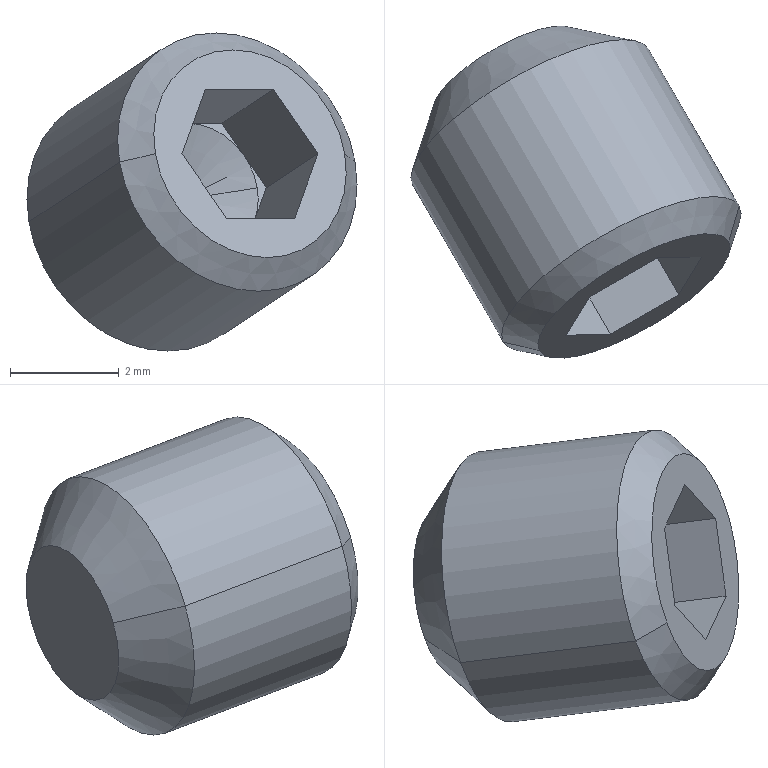Part | SolidWorks | features BaseBody 1 | 1 solid | 22 faces | box 6.067 x 6.109 x 5.848 mm | volume 77.596 mm3 | plane 14 | cone 6 | cylinder 2 | commonest cylinder face diameters 5 x2
STEP:
#1=CARTESIAN_POINT('',(451.556,1814.827,-1176.378));
#2=VERTEX_POINT('',#1);
#3=CARTESIAN_POINT('',(447.226,1812.327,-1176.378));
#4=VERTEX_POINT('',#3);
#5=CARTESIAN_POINT('',(449.391,1813.577,-1176.378));
#6=DIRECTION('',(0.4749,-0.8225,0.3132));
#7=DIRECTION('',(0.866,0.5,0.));
#8=AXIS2_PLACEMENT_3D('',#5,#6,#7);
#9=CIRCLE('',#8,2.5);
#10=EDGE_CURVE('',#2,#4,#9,.T.);
#11=ORIENTED_EDGE('',*,*,#10,.T.);
#12=CARTESIAN_POINT('',(448.893,1809.44,-1175.279));
#13=VERTEX_POINT('',#12);
#14=CARTESIAN_POINT('',(449.126,1809.037,-1175.125));
#15=DIRECTION('',(0.4749,-0.8225,0.3132));
#16=VECTOR('',#15,1000.);
#17=LINE('',#14,#16);
#18=EDGE_CURVE('',#4,#13,#17,.T.);
#19=ORIENTED_EDGE('',*,*,#18,.T.);
#20=CARTESIAN_POINT('',(453.223,1811.94,-1175.279));
#21=VERTEX_POINT('',#20);
#22=CARTESIAN_POINT('',(451.058,1810.69,-1175.279));
#23=DIRECTION('',(-0.4749,0.8225,-0.3132));
#24=DIRECTION('',(0.866,0.5,0.));
#25=AXIS2_PLACEMENT_3D('',#22,#23,#24);
#26=CIRCLE('',#25,2.5);
#27=EDGE_CURVE('',#13,#21,#26,.T.);
#28=ORIENTED_EDGE('',*,*,#27,.T.);
#29=CARTESIAN_POINT('',(453.456,1811.537,-1175.125));
#30=DIRECTION('',(0.4749,-0.8225,0.3132));
#31=VECTOR('',#30,1000.);
#32=LINE('',#29,#31);
#33=EDGE_CURVE('',#2,#21,#32,.T.);
#34=ORIENTED_EDGE('',*,*,#33,.F.);
#35=EDGE_LOOP('',(#11,#19,#28,#34));
#36=FACE_OUTER_BOUND('',#35,.T.);
#37=CARTESIAN_POINT('',(451.291,1810.287,-1175.125));
#38=DIRECTION('',(0.4749,-0.8225,0.3132));
#39=DIRECTION('',(0.866,0.5,0.));
#40=AXIS2_PLACEMENT_3D('',#37,#38,#39);
#41=CYLINDRICAL_SURFACE('',#40,2.5);
#42=ADVANCED_FACE('',(#36),#41,.T.);
#43=CARTESIAN_POINT('',(449.55,1809.282,-1175.125));
#44=VERTEX_POINT('',#43);
#45=CARTESIAN_POINT('',(453.031,1811.292,-1175.125));
#46=VERTEX_POINT('',#45);
#47=CARTESIAN_POINT('',(451.291,1810.287,-1175.125));
#48=DIRECTION('',(-0.4749,0.8225,-0.3132));
#49=DIRECTION('',(-0.866,-0.5,0.));
#50=AXIS2_PLACEMENT_3D('',#47,#48,#49);
#51=CIRCLE('',#50,2.009);
#52=EDGE_CURVE('',#44,#46,#51,.T.);
#53=ORIENTED_EDGE('',*,*,#52,.T.);
#54=CARTESIAN_POINT('',(453.223,1811.94,-1175.279));
#55=DIRECTION('',(0.2766,0.9351,-0.2214));
#56=VECTOR('',#55,1000.);
#57=LINE('',#54,#56);
#58=EDGE_CURVE('',#46,#21,#57,.T.);
#59=ORIENTED_EDGE('',*,*,#58,.T.);
#60=ORIENTED_EDGE('',*,*,#27,.F.);
#61=CARTESIAN_POINT('',(448.893,1809.44,-1175.279));
#62=DIRECTION('',(-0.9481,0.228,-0.2214));
#63=VECTOR('',#62,1000.);
#64=LINE('',#61,#63);
#65=EDGE_CURVE('',#44,#13,#64,.T.);
#66=ORIENTED_EDGE('',*,*,#65,.F.);
#67=EDGE_LOOP('',(#53,#59,#60,#66));
#68=FACE_OUTER_BOUND('',#67,.T.);
#69=CARTESIAN_POINT('',(451.058,1810.69,-1175.279));
#70=DIRECTION('',(-0.4749,0.8225,-0.3132));
#71=DIRECTION('',(-0.866,-0.5,0.));
#72=AXIS2_PLACEMENT_3D('',#69,#70,#71);
#73=CONICAL_SURFACE('',#72,2.5,0.7854);
#74=ADVANCED_FACE('',(#68),#73,.T.);
#75=CARTESIAN_POINT('',(450.216,1815.149,-1176.691));
#76=VERTEX_POINT('',#75);
#77=CARTESIAN_POINT('',(447.617,1813.649,-1176.691));
#78=VERTEX_POINT('',#77);
#79=CARTESIAN_POINT('',(448.916,1814.399,-1176.691));
#80=DIRECTION('',(0.4749,-0.8225,0.3132));
#81=DIRECTION('',(0.866,0.5,0.));
#82=AXIS2_PLACEMENT_3D('',#79,#80,#81);
#83=CIRCLE('',#82,1.5);
#84=EDGE_CURVE('',#76,#78,#83,.T.);
#85=ORIENTED_EDGE('',*,*,#84,.T.);
#86=CARTESIAN_POINT('',(447.226,1812.327,-1176.378));
#87=DIRECTION('',(-0.2766,-0.9351,0.2214));
#88=VECTOR('',#87,1000.);
#89=LINE('',#86,#88);
#90=EDGE_CURVE('',#78,#4,#89,.T.);
#91=ORIENTED_EDGE('',*,*,#90,.T.);
#92=ORIENTED_EDGE('',*,*,#10,.F.);
#93=CARTESIAN_POINT('',(451.556,1814.827,-1176.378));
#94=DIRECTION('',(0.9481,-0.228,0.2214));
#95=VECTOR('',#94,1000.);
#96=LINE('',#93,#95);
#97=EDGE_CURVE('',#76,#2,#96,.T.);
#98=ORIENTED_EDGE('',*,*,#97,.F.);
#99=EDGE_LOOP('',(#85,#91,#92,#98));
#100=FACE_OUTER_BOUND('',#99,.T.);
#101=CARTESIAN_POINT('',(449.391,1813.577,-1176.378));
#102=DIRECTION('',(0.4749,-0.8225,0.3132));
#103=DIRECTION('',(0.866,0.5,0.));
#104=AXIS2_PLACEMENT_3D('',#101,#102,#103);
#105=CONICAL_SURFACE('',#104,2.5,0.7854);
#106=ADVANCED_FACE('',(#100),#105,.T.);
#107=CARTESIAN_POINT('',(449.998,1812.525,-1175.978));
#108=VERTEX_POINT('',#107);
#109=CARTESIAN_POINT('',(451.424,1812.557,-1175.752));
#110=VERTEX_POINT('',#109);
#111=CARTESIAN_POINT('',(451.424,1812.557,-1175.752));
#112=DIRECTION('',(0.9874,0.02178,0.1566));
#113=VECTOR('',#112,1000.);
#114=LINE('',#111,#113);
#115=EDGE_CURVE('',#108,#110,#114,.T.);
#116=ORIENTED_EDGE('',*,*,#115,.F.);
#117=CARTESIAN_POINT('',(449.258,1811.307,-1175.752));
#118=VERTEX_POINT('',#117);
#119=CARTESIAN_POINT('',(449.258,1811.307,-1175.752));
#120=DIRECTION('',(-0.5126,-0.8442,0.1566));
#121=VECTOR('',#120,1000.);
#122=LINE('',#119,#121);
#123=EDGE_CURVE('',#108,#118,#122,.T.);
#124=ORIENTED_EDGE('',*,*,#123,.T.);
#125=CARTESIAN_POINT('',(449.501,1811.221,-1176.345));
#126=VERTEX_POINT('',#125);
#127=CARTESIAN_POINT('',(450.341,1811.932,-1175.752));
#128=DIRECTION('',(-0.4749,0.8225,-0.3132));
#129=DIRECTION('',(0.866,0.5,0.));
#130=AXIS2_PLACEMENT_3D('',#127,#128,#129);
#131=CIRCLE('',#130,1.25);
#132=EDGE_CURVE('',#126,#118,#131,.T.);
#133=ORIENTED_EDGE('',*,*,#132,.F.);
#134=CARTESIAN_POINT('',(450.537,1811.593,-1176.939));
#135=VERTEX_POINT('',#134);
#136=CARTESIAN_POINT('',(450.341,1811.932,-1175.752));
#137=DIRECTION('',(-0.4749,0.8225,-0.3132));
#138=DIRECTION('',(0.866,0.5,0.));
#139=AXIS2_PLACEMENT_3D('',#136,#137,#138);
#140=CIRCLE('',#139,1.25);
#141=EDGE_CURVE('',#135,#126,#140,.T.);
#142=ORIENTED_EDGE('',*,*,#141,.F.);
#143=CARTESIAN_POINT('',(451.376,1812.304,-1176.345));
#144=VERTEX_POINT('',#143);
#145=CARTESIAN_POINT('',(450.341,1811.932,-1175.752));
#146=DIRECTION('',(-0.4749,0.8225,-0.3132));
#147=DIRECTION('',(0.866,0.5,0.));
#148=AXIS2_PLACEMENT_3D('',#145,#146,#147);
#149=CIRCLE('',#148,1.25);
#150=EDGE_CURVE('',#144,#135,#149,.T.);
#151=ORIENTED_EDGE('',*,*,#150,.F.);
#152=CARTESIAN_POINT('',(450.341,1811.932,-1175.752));
#153=DIRECTION('',(-0.4749,0.8225,-0.3132));
#154=DIRECTION('',(0.866,0.5,0.));
#155=AXIS2_PLACEMENT_3D('',#152,#153,#154);
#156=CIRCLE('',#155,1.25);
#157=EDGE_CURVE('',#110,#144,#156,.T.);
#158=ORIENTED_EDGE('',*,*,#157,.F.);
#159=EDGE_LOOP('',(#116,#124,#133,#142,#151,#158));
#160=FACE_OUTER_BOUND('',#159,.T.);
#161=CARTESIAN_POINT('',(450.341,1811.932,-1175.752));
#162=DIRECTION('',(0.4749,-0.8225,0.3132));
#163=DIRECTION('',(0.866,0.5,0.));
#164=AXIS2_PLACEMENT_3D('',#161,#162,#163);
#165=CONICAL_SURFACE('',#164,1.25,1.047);
#166=ADVANCED_FACE('',(#160),#165,.F.);
#167=ORIENTED_EDGE('',*,*,#18,.F.);
#168=CARTESIAN_POINT('',(449.391,1813.577,-1176.378));
#169=DIRECTION('',(0.4749,-0.8225,0.3132));
#170=DIRECTION('',(0.866,0.5,0.));
#171=AXIS2_PLACEMENT_3D('',#168,#169,#170);
#172=CIRCLE('',#171,2.5);
#173=EDGE_CURVE('',#4,#2,#172,.T.);
#174=ORIENTED_EDGE('',*,*,#173,.T.);
#175=ORIENTED_EDGE('',*,*,#33,.T.);
#176=CARTESIAN_POINT('',(451.058,1810.69,-1175.279));
#177=DIRECTION('',(-0.4749,0.8225,-0.3132));
#178=DIRECTION('',(0.866,0.5,0.));
#179=AXIS2_PLACEMENT_3D('',#176,#177,#178);
#180=CIRCLE('',#179,2.5);
#181=EDGE_CURVE('',#21,#13,#180,.T.);
#182=ORIENTED_EDGE('',*,*,#181,.T.);
#183=EDGE_LOOP('',(#167,#174,#175,#182));
#184=FACE_OUTER_BOUND('',#183,.T.);
#185=CARTESIAN_POINT('',(451.291,1810.287,-1175.125));
#186=DIRECTION('',(0.4749,-0.8225,0.3132));
#187=DIRECTION('',(0.866,0.5,0.));
#188=AXIS2_PLACEMENT_3D('',#185,#186,#187);
#189=CYLINDRICAL_SURFACE('',#188,2.5);
#190=ADVANCED_FACE('',(#184),#189,.T.);
#191=ORIENTED_EDGE('',*,*,#58,.F.);
#192=CARTESIAN_POINT('',(451.291,1810.287,-1175.125));
#193=DIRECTION('',(-0.4749,0.8225,-0.3132));
#194=DIRECTION('',(-0.866,-0.5,0.));
#195=AXIS2_PLACEMENT_3D('',#192,#193,#194);
#196=CIRCLE('',#195,2.009);
#197=EDGE_CURVE('',#46,#44,#196,.T.);
#198=ORIENTED_EDGE('',*,*,#197,.T.);
#199=ORIENTED_EDGE('',*,*,#65,.T.);
#200=ORIENTED_EDGE('',*,*,#181,.F.);
#201=EDGE_LOOP('',(#191,#198,#199,#200));
#202=FACE_OUTER_BOUND('',#201,.T.);
#203=CARTESIAN_POINT('',(451.058,1810.69,-1175.279));
#204=DIRECTION('',(-0.4749,0.8225,-0.3132));
#205=DIRECTION('',(-0.866,-0.5,0.));
#206=AXIS2_PLACEMENT_3D('',#203,#204,#205);
#207=CONICAL_SURFACE('',#206,2.5,0.7854);
#208=ADVANCED_FACE('',(#202),#207,.T.);
#209=ORIENTED_EDGE('',*,*,#90,.F.);
#210=CARTESIAN_POINT('',(448.916,1814.399,-1176.691));
#211=DIRECTION('',(0.4749,-0.8225,0.3132));
#212=DIRECTION('',(0.866,0.5,0.));
#213=AXIS2_PLACEMENT_3D('',#210,#211,#212);
#214=CIRCLE('',#213,1.5);
#215=EDGE_CURVE('',#78,#76,#214,.T.);
#216=ORIENTED_EDGE('',*,*,#215,.T.);
#217=ORIENTED_EDGE('',*,*,#97,.T.);
#218=ORIENTED_EDGE('',*,*,#173,.F.);
#219=EDGE_LOOP('',(#209,#216,#217,#218));
#220=FACE_OUTER_BOUND('',#219,.T.);
#221=CARTESIAN_POINT('',(449.391,1813.577,-1176.378));
#222=DIRECTION('',(0.4749,-0.8225,0.3132));
#223=DIRECTION('',(0.866,0.5,0.));
#224=AXIS2_PLACEMENT_3D('',#221,#222,#223);
#225=CONICAL_SURFACE('',#224,2.5,0.7854);
#226=ADVANCED_FACE('',(#220),#225,.T.);
#227=CARTESIAN_POINT('',(450.861,1809.587,-1176.312));
#228=VERTEX_POINT('',#227);
#229=CARTESIAN_POINT('',(452.111,1810.309,-1176.312));
#230=VERTEX_POINT('',#229);
#231=CARTESIAN_POINT('',(453.227,1810.953,-1176.312));
#232=DIRECTION('',(0.866,0.5,0.));
#233=VECTOR('',#232,1000.);
#234=LINE('',#231,#233);
#235=EDGE_CURVE('',#228,#230,#234,.T.);
#236=ORIENTED_EDGE('',*,*,#235,.F.);
#237=CARTESIAN_POINT('',(450.041,1809.565,-1175.125));
#238=VERTEX_POINT('',#237);
#239=CARTESIAN_POINT('',(450.041,1809.565,-1175.125));
#240=DIRECTION('',(0.5686,0.01513,-0.8225));
#241=VECTOR('',#240,1000.);
#242=LINE('',#239,#241);
#243=EDGE_CURVE('',#238,#228,#242,.T.);
#244=ORIENTED_EDGE('',*,*,#243,.F.);
#245=CARTESIAN_POINT('',(450.47,1810.265,-1173.938));
#246=VERTEX_POINT('',#245);
#247=CARTESIAN_POINT('',(450.47,1810.265,-1173.938));
#248=DIRECTION('',(-0.2974,-0.4849,-0.8225));
#249=VECTOR('',#248,1000.);
#250=LINE('',#247,#249);
#251=EDGE_CURVE('',#246,#238,#250,.T.);
#252=ORIENTED_EDGE('',*,*,#251,.F.);
#253=CARTESIAN_POINT('',(451.72,1810.987,-1173.938));
#254=VERTEX_POINT('',#253);
#255=CARTESIAN_POINT('',(452.835,1811.631,-1173.938));
#256=DIRECTION('',(-0.866,-0.5,0.));
#257=VECTOR('',#256,1000.);
#258=LINE('',#255,#257);
#259=EDGE_CURVE('',#254,#246,#258,.T.);
#260=ORIENTED_EDGE('',*,*,#259,.F.);
#261=CARTESIAN_POINT('',(452.541,1811.009,-1175.125));
#262=VERTEX_POINT('',#261);
#263=CARTESIAN_POINT('',(452.541,1811.009,-1175.125));
#264=DIRECTION('',(-0.5686,-0.01513,0.8225));
#265=VECTOR('',#264,1000.);
#266=LINE('',#263,#265);
#267=EDGE_CURVE('',#262,#254,#266,.T.);
#268=ORIENTED_EDGE('',*,*,#267,.F.);
#269=CARTESIAN_POINT('',(452.111,1810.309,-1176.312));
#270=DIRECTION('',(0.2974,0.4849,0.8225));
#271=VECTOR('',#270,1000.);
#272=LINE('',#269,#271);
#273=EDGE_CURVE('',#230,#262,#272,.T.);
#274=ORIENTED_EDGE('',*,*,#273,.F.);
#275=EDGE_LOOP('',(#236,#244,#252,#260,#268,#274));
#276=FACE_BOUND('',#275,.T.);
#277=ORIENTED_EDGE('',*,*,#52,.F.);
#278=ORIENTED_EDGE('',*,*,#197,.F.);
#279=EDGE_LOOP('',(#277,#278));
#280=FACE_OUTER_BOUND('',#279,.T.);
#281=CARTESIAN_POINT('',(453.031,1811.292,-1175.125));
#282=DIRECTION('',(-0.4749,0.8225,-0.3132));
#283=DIRECTION('',(-0.866,-0.5,0.));
#284=AXIS2_PLACEMENT_3D('',#281,#282,#283);
#285=PLANE('',#284);
#286=ADVANCED_FACE('',(#276,#280),#285,.F.);
#287=ORIENTED_EDGE('',*,*,#84,.F.);
#288=ORIENTED_EDGE('',*,*,#215,.F.);
#289=EDGE_LOOP('',(#287,#288));
#290=FACE_OUTER_BOUND('',#289,.T.);
#291=CARTESIAN_POINT('',(448.916,1814.399,-1176.691));
#292=DIRECTION('',(0.4749,-0.8225,0.3132));
#293=DIRECTION('',(0.866,0.5,0.));
#294=AXIS2_PLACEMENT_3D('',#291,#292,#293);
#295=PLANE('',#294);
#296=ADVANCED_FACE('',(#290),#295,.F.);
#297=CARTESIAN_POINT('',(451.591,1812.654,-1175.752));
#298=VERTEX_POINT('',#297);
#299=CARTESIAN_POINT('',(451.376,1812.304,-1176.345));
#300=DIRECTION('',(0.2974,0.4849,0.8225));
#301=VECTOR('',#300,1000.);
#302=LINE('',#299,#301);
#303=EDGE_CURVE('',#144,#298,#302,.T.);
#304=ORIENTED_EDGE('',*,*,#303,.F.);
#305=CARTESIAN_POINT('',(451.162,1811.954,-1176.939));
#306=VERTEX_POINT('',#305);
#307=CARTESIAN_POINT('',(451.162,1811.954,-1176.939));
#308=DIRECTION('',(0.2974,0.4849,0.8225));
#309=VECTOR('',#308,1000.);
#310=LINE('',#307,#309);
#311=EDGE_CURVE('',#306,#144,#310,.T.);
#312=ORIENTED_EDGE('',*,*,#311,.F.);
#313=CARTESIAN_POINT('',(452.111,1810.309,-1176.312));
#314=DIRECTION('',(-0.4749,0.8225,-0.3132));
#315=VECTOR('',#314,1000.);
#316=LINE('',#313,#315);
#317=EDGE_CURVE('',#230,#306,#316,.T.);
#318=ORIENTED_EDGE('',*,*,#317,.F.);
#319=ORIENTED_EDGE('',*,*,#273,.T.);
#320=CARTESIAN_POINT('',(451.591,1812.654,-1175.752));
#321=DIRECTION('',(0.4749,-0.8225,0.3132));
#322=VECTOR('',#321,1000.);
#323=LINE('',#320,#322);
#324=EDGE_CURVE('',#298,#262,#323,.T.);
#325=ORIENTED_EDGE('',*,*,#324,.F.);
#326=EDGE_LOOP('',(#304,#312,#318,#319,#325));
#327=FACE_OUTER_BOUND('',#326,.T.);
#328=CARTESIAN_POINT('',(451.162,1811.954,-1176.939));
#329=DIRECTION('',(0.8283,0.2974,-0.4749));
#330=DIRECTION('',(-0.4974,0.,-0.8675));
#331=AXIS2_PLACEMENT_3D('',#328,#329,#330);
#332=PLANE('',#331);
#333=ADVANCED_FACE('',(#327),#332,.F.);
#334=CARTESIAN_POINT('',(450.537,1811.593,-1176.939));
#335=DIRECTION('',(0.866,0.5,0.));
#336=VECTOR('',#335,1000.);
#337=LINE('',#334,#336);
#338=EDGE_CURVE('',#135,#306,#337,.T.);
#339=ORIENTED_EDGE('',*,*,#338,.F.);
#340=CARTESIAN_POINT('',(449.912,1811.232,-1176.939));
#341=VERTEX_POINT('',#340);
#342=CARTESIAN_POINT('',(449.912,1811.232,-1176.939));
#343=DIRECTION('',(0.866,0.5,0.));
#344=VECTOR('',#343,1000.);
#345=LINE('',#342,#344);
#346=EDGE_CURVE('',#341,#135,#345,.T.);
#347=ORIENTED_EDGE('',*,*,#346,.F.);
#348=CARTESIAN_POINT('',(450.861,1809.587,-1176.312));
#349=DIRECTION('',(-0.4749,0.8225,-0.3132));
#350=VECTOR('',#349,1000.);
#351=LINE('',#348,#350);
#352=EDGE_CURVE('',#228,#341,#351,.T.);
#353=ORIENTED_EDGE('',*,*,#352,.F.);
#354=ORIENTED_EDGE('',*,*,#235,.T.);
#355=ORIENTED_EDGE('',*,*,#317,.T.);
#356=EDGE_LOOP('',(#339,#347,#353,#354,#355));
#357=FACE_OUTER_BOUND('',#356,.T.);
#358=CARTESIAN_POINT('',(449.912,1811.232,-1176.939));
#359=DIRECTION('',(0.1566,-0.2712,-0.9497));
#360=DIRECTION('',(0.,0.9616,-0.2746));
#361=AXIS2_PLACEMENT_3D('',#358,#359,#360);
#362=PLANE('',#361);
#363=ADVANCED_FACE('',(#357),#362,.F.);
#364=CARTESIAN_POINT('',(449.501,1811.221,-1176.345));
#365=DIRECTION('',(0.5686,0.01513,-0.8225));
#366=VECTOR('',#365,1000.);
#367=LINE('',#364,#366);
#368=EDGE_CURVE('',#126,#341,#367,.T.);
#369=ORIENTED_EDGE('',*,*,#368,.F.);
#370=CARTESIAN_POINT('',(449.091,1811.21,-1175.752));
#371=VERTEX_POINT('',#370);
#372=CARTESIAN_POINT('',(449.091,1811.21,-1175.752));
#373=DIRECTION('',(0.5686,0.01513,-0.8225));
#374=VECTOR('',#373,1000.);
#375=LINE('',#372,#374);
#376=EDGE_CURVE('',#371,#126,#375,.T.);
#377=ORIENTED_EDGE('',*,*,#376,.F.);
#378=CARTESIAN_POINT('',(450.041,1809.565,-1175.125));
#379=DIRECTION('',(-0.4749,0.8225,-0.3132));
#380=VECTOR('',#379,1000.);
#381=LINE('',#378,#380);
#382=EDGE_CURVE('',#238,#371,#381,.T.);
#383=ORIENTED_EDGE('',*,*,#382,.F.);
#384=ORIENTED_EDGE('',*,*,#243,.T.);
#385=ORIENTED_EDGE('',*,*,#352,.T.);
#386=EDGE_LOOP('',(#369,#377,#383,#384,#385));
#387=FACE_OUTER_BOUND('',#386,.T.);
#388=CARTESIAN_POINT('',(449.091,1811.21,-1175.752));
#389=DIRECTION('',(-0.6717,-0.5686,-0.4749));
#390=DIRECTION('',(0.6461,-0.7633,0.));
#391=AXIS2_PLACEMENT_3D('',#388,#389,#390);
#392=PLANE('',#391);
#393=ADVANCED_FACE('',(#387),#392,.F.);
#394=CARTESIAN_POINT('',(449.306,1811.56,-1175.158));
#395=VERTEX_POINT('',#394);
#396=CARTESIAN_POINT('',(449.306,1811.56,-1175.158));
#397=DIRECTION('',(-0.2974,-0.4849,-0.8225));
#398=VECTOR('',#397,1000.);
#399=LINE('',#396,#398);
#400=EDGE_CURVE('',#395,#371,#399,.T.);
#401=ORIENTED_EDGE('',*,*,#400,.F.);
#402=CARTESIAN_POINT('',(449.52,1811.91,-1174.564));
#403=VERTEX_POINT('',#402);
#404=CARTESIAN_POINT('',(449.52,1811.91,-1174.564));
#405=DIRECTION('',(-0.2974,-0.4849,-0.8225));
#406=VECTOR('',#405,1000.);
#407=LINE('',#404,#406);
#408=EDGE_CURVE('',#403,#395,#407,.T.);
#409=ORIENTED_EDGE('',*,*,#408,.F.);
#410=CARTESIAN_POINT('',(450.47,1810.265,-1173.938));
#411=DIRECTION('',(-0.4749,0.8225,-0.3132));
#412=VECTOR('',#411,1000.);
#413=LINE('',#410,#412);
#414=EDGE_CURVE('',#246,#403,#413,.T.);
#415=ORIENTED_EDGE('',*,*,#414,.F.);
#416=ORIENTED_EDGE('',*,*,#251,.T.);
#417=ORIENTED_EDGE('',*,*,#382,.T.);
#418=EDGE_LOOP('',(#401,#409,#415,#416,#417));
#419=FACE_OUTER_BOUND('',#418,.T.);
#420=CARTESIAN_POINT('',(449.52,1811.91,-1174.564));
#421=DIRECTION('',(-0.8283,-0.2974,0.4749));
#422=DIRECTION('',(0.4974,0.,0.8675));
#423=AXIS2_PLACEMENT_3D('',#420,#421,#422);
#424=PLANE('',#423);
#425=ADVANCED_FACE('',(#419),#424,.F.);
#426=CARTESIAN_POINT('',(450.145,1812.271,-1174.564));
#427=VERTEX_POINT('',#426);
#428=CARTESIAN_POINT('',(450.145,1812.271,-1174.564));
#429=DIRECTION('',(-0.866,-0.5,0.));
#430=VECTOR('',#429,1000.);
#431=LINE('',#428,#430);
#432=EDGE_CURVE('',#427,#403,#431,.T.);
#433=ORIENTED_EDGE('',*,*,#432,.F.);
#434=CARTESIAN_POINT('',(450.77,1812.632,-1174.564));
#435=VERTEX_POINT('',#434);
#436=CARTESIAN_POINT('',(450.77,1812.632,-1174.564));
#437=DIRECTION('',(-0.866,-0.5,0.));
#438=VECTOR('',#437,1000.);
#439=LINE('',#436,#438);
#440=EDGE_CURVE('',#435,#427,#439,.T.);
#441=ORIENTED_EDGE('',*,*,#440,.F.);
#442=CARTESIAN_POINT('',(451.72,1810.987,-1173.938));
#443=DIRECTION('',(-0.4749,0.8225,-0.3132));
#444=VECTOR('',#443,1000.);
#445=LINE('',#442,#444);
#446=EDGE_CURVE('',#254,#435,#445,.T.);
#447=ORIENTED_EDGE('',*,*,#446,.F.);
#448=ORIENTED_EDGE('',*,*,#259,.T.);
#449=ORIENTED_EDGE('',*,*,#414,.T.);
#450=EDGE_LOOP('',(#433,#441,#447,#448,#449));
#451=FACE_OUTER_BOUND('',#450,.T.);
#452=CARTESIAN_POINT('',(450.77,1812.632,-1174.564));
#453=DIRECTION('',(-0.1566,0.2712,0.9497));
#454=DIRECTION('',(0.,-0.9616,0.2746));
#455=AXIS2_PLACEMENT_3D('',#452,#453,#454);
#456=PLANE('',#455);
#457=ADVANCED_FACE('',(#451),#456,.F.);
#458=CARTESIAN_POINT('',(451.181,1812.643,-1175.158));
#459=VERTEX_POINT('',#458);
#460=CARTESIAN_POINT('',(451.181,1812.643,-1175.158));
#461=DIRECTION('',(-0.5686,-0.01513,0.8225));
#462=VECTOR('',#461,1000.);
#463=LINE('',#460,#462);
#464=EDGE_CURVE('',#459,#435,#463,.T.);
#465=ORIENTED_EDGE('',*,*,#464,.F.);
#466=CARTESIAN_POINT('',(451.591,1812.654,-1175.752));
#467=DIRECTION('',(-0.5686,-0.01513,0.8225));
#468=VECTOR('',#467,1000.);
#469=LINE('',#466,#468);
#470=EDGE_CURVE('',#298,#459,#469,.T.);
#471=ORIENTED_EDGE('',*,*,#470,.F.);
#472=ORIENTED_EDGE('',*,*,#324,.T.);
#473=ORIENTED_EDGE('',*,*,#267,.T.);
#474=ORIENTED_EDGE('',*,*,#446,.T.);
#475=EDGE_LOOP('',(#465,#471,#472,#473,#474));
#476=FACE_OUTER_BOUND('',#475,.T.);
#477=CARTESIAN_POINT('',(451.591,1812.654,-1175.752));
#478=DIRECTION('',(0.6717,0.5686,0.4749));
#479=DIRECTION('',(-0.6461,0.7633,0.));
#480=AXIS2_PLACEMENT_3D('',#477,#478,#479);
#481=PLANE('',#480);
#482=ADVANCED_FACE('',(#476),#481,.F.);
#483=ORIENTED_EDGE('',*,*,#470,.T.);
#484=CARTESIAN_POINT('',(450.341,1811.932,-1175.752));
#485=DIRECTION('',(-0.4749,0.8225,-0.3132));
#486=DIRECTION('',(0.866,0.5,0.));
#487=AXIS2_PLACEMENT_3D('',#484,#485,#486);
#488=CIRCLE('',#487,1.25);
#489=EDGE_CURVE('',#459,#110,#488,.T.);
#490=ORIENTED_EDGE('',*,*,#489,.T.);
#491=ORIENTED_EDGE('',*,*,#157,.T.);
#492=ORIENTED_EDGE('',*,*,#303,.T.);
#493=EDGE_LOOP('',(#483,#490,#491,#492));
#494=FACE_OUTER_BOUND('',#493,.T.);
#495=CARTESIAN_POINT('',(450.341,1811.932,-1175.752));
#496=DIRECTION('',(0.4749,-0.8225,0.3132));
#497=DIRECTION('',(0.866,0.5,0.));
#498=AXIS2_PLACEMENT_3D('',#495,#496,#497);
#499=PLANE('',#498);
#500=ADVANCED_FACE('',(#494),#499,.T.);
#501=ORIENTED_EDGE('',*,*,#311,.T.);
#502=ORIENTED_EDGE('',*,*,#150,.T.);
#503=ORIENTED_EDGE('',*,*,#338,.T.);
#504=EDGE_LOOP('',(#501,#502,#503));
#505=FACE_OUTER_BOUND('',#504,.T.);
#506=CARTESIAN_POINT('',(450.341,1811.932,-1175.752));
#507=DIRECTION('',(0.4749,-0.8225,0.3132));
#508=DIRECTION('',(0.866,0.5,0.));
#509=AXIS2_PLACEMENT_3D('',#506,#507,#508);
#510=PLANE('',#509);
#511=ADVANCED_FACE('',(#505),#510,.T.);
#512=ORIENTED_EDGE('',*,*,#346,.T.);
#513=ORIENTED_EDGE('',*,*,#141,.T.);
#514=ORIENTED_EDGE('',*,*,#368,.T.);
#515=EDGE_LOOP('',(#512,#513,#514));
#516=FACE_OUTER_BOUND('',#515,.T.);
#517=CARTESIAN_POINT('',(450.341,1811.932,-1175.752));
#518=DIRECTION('',(0.4749,-0.8225,0.3132));
#519=DIRECTION('',(0.866,0.5,0.));
#520=AXIS2_PLACEMENT_3D('',#517,#518,#519);
#521=PLANE('',#520);
#522=ADVANCED_FACE('',(#516),#521,.T.);
#523=ORIENTED_EDGE('',*,*,#376,.T.);
#524=ORIENTED_EDGE('',*,*,#132,.T.);
#525=CARTESIAN_POINT('',(450.341,1811.932,-1175.752));
#526=DIRECTION('',(-0.4749,0.8225,-0.3132));
#527=DIRECTION('',(0.866,0.5,0.));
#528=AXIS2_PLACEMENT_3D('',#525,#526,#527);
#529=CIRCLE('',#528,1.25);
#530=EDGE_CURVE('',#118,#395,#529,.T.);
#531=ORIENTED_EDGE('',*,*,#530,.T.);
#532=ORIENTED_EDGE('',*,*,#400,.T.);
#533=EDGE_LOOP('',(#523,#524,#531,#532));
#534=FACE_OUTER_BOUND('',#533,.T.);
#535=CARTESIAN_POINT('',(450.341,1811.932,-1175.752));
#536=DIRECTION('',(0.4749,-0.8225,0.3132));
#537=DIRECTION('',(0.866,0.5,0.));
#538=AXIS2_PLACEMENT_3D('',#535,#536,#537);
#539=PLANE('',#538);
#540=ADVANCED_FACE('',(#534),#539,.T.);
#541=ORIENTED_EDGE('',*,*,#408,.T.);
#542=CARTESIAN_POINT('',(450.341,1811.932,-1175.752));
#543=DIRECTION('',(-0.4749,0.8225,-0.3132));
#544=DIRECTION('',(0.866,0.5,0.));
#545=AXIS2_PLACEMENT_3D('',#542,#543,#544);
#546=CIRCLE('',#545,1.25);
#547=EDGE_CURVE('',#395,#427,#546,.T.);
#548=ORIENTED_EDGE('',*,*,#547,.T.);
#549=ORIENTED_EDGE('',*,*,#432,.T.);
#550=EDGE_LOOP('',(#541,#548,#549));
#551=FACE_OUTER_BOUND('',#550,.T.);
#552=CARTESIAN_POINT('',(450.341,1811.932,-1175.752));
#553=DIRECTION('',(0.4749,-0.8225,0.3132));
#554=DIRECTION('',(0.866,0.5,0.));
#555=AXIS2_PLACEMENT_3D('',#552,#553,#554);
#556=PLANE('',#555);
#557=ADVANCED_FACE('',(#551),#556,.T.);
#558=ORIENTED_EDGE('',*,*,#440,.T.);
#559=CARTESIAN_POINT('',(450.341,1811.932,-1175.752));
#560=DIRECTION('',(-0.4749,0.8225,-0.3132));
#561=DIRECTION('',(0.866,0.5,0.));
#562=AXIS2_PLACEMENT_3D('',#559,#560,#561);
#563=CIRCLE('',#562,1.25);
#564=EDGE_CURVE('',#427,#459,#563,.T.);
#565=ORIENTED_EDGE('',*,*,#564,.T.);
#566=ORIENTED_EDGE('',*,*,#464,.T.);
#567=EDGE_LOOP('',(#558,#565,#566));
#568=FACE_OUTER_BOUND('',#567,.T.);
#569=CARTESIAN_POINT('',(450.341,1811.932,-1175.752));
#570=DIRECTION('',(0.4749,-0.8225,0.3132));
#571=DIRECTION('',(0.866,0.5,0.));
#572=AXIS2_PLACEMENT_3D('',#569,#570,#571);
#573=PLANE('',#572);
#574=ADVANCED_FACE('',(#568),#573,.T.);
#575=ORIENTED_EDGE('',*,*,#123,.F.);
#576=ORIENTED_EDGE('',*,*,#115,.T.);
#577=ORIENTED_EDGE('',*,*,#489,.F.);
#578=ORIENTED_EDGE('',*,*,#564,.F.);
#579=ORIENTED_EDGE('',*,*,#547,.F.);
#580=ORIENTED_EDGE('',*,*,#530,.F.);
#581=EDGE_LOOP('',(#575,#576,#577,#578,#579,#580));
#582=FACE_OUTER_BOUND('',#581,.T.);
#583=CARTESIAN_POINT('',(450.341,1811.932,-1175.752));
#584=DIRECTION('',(0.4749,-0.8225,0.3132));
#585=DIRECTION('',(0.866,0.5,0.));
#586=AXIS2_PLACEMENT_3D('',#583,#584,#585);
#587=CONICAL_SURFACE('',#586,1.25,1.047);
#588=ADVANCED_FACE('',(#582),#587,.F.);
#589=CLOSED_SHELL('',(#42,#74,#106,#166,#190,#208,#226,#286,#296,#333,#363,#393,#425,#457,#482,#500,#511,#522,#540,#557,#574,#588));
#590=MANIFOLD_SOLID_BREP('',#589);
#591=CARTESIAN_POINT('',(0.,0.,0.));
#592=DIRECTION('',(0.,0.,1.));
#593=DIRECTION('',(1.,0.,0.));
#594=AXIS2_PLACEMENT_3D('',#591,#592,#593);
#595=(LENGTH_UNIT()NAMED_UNIT(*)SI_UNIT(.MILLI.,.METRE.));
#596=UNCERTAINTY_MEASURE_WITH_UNIT(LENGTH_MEASURE(0.00001),#595,'','');
#597=(NAMED_UNIT(*)PLANE_ANGLE_UNIT()SI_UNIT($,.RADIAN.));
#598=(NAMED_UNIT(*)SI_UNIT($,.STERADIAN.)SOLID_ANGLE_UNIT());
#599=(GEOMETRIC_REPRESENTATION_CONTEXT(3)GLOBAL_UNCERTAINTY_ASSIGNED_CONTEXT((#596))GLOBAL_UNIT_ASSIGNED_CONTEXT((#595,#597,#598))REPRESENTATION_CONTEXT('',''));
#600=ADVANCED_BREP_SHAPE_REPRESENTATION('',(#590,#594),#599);